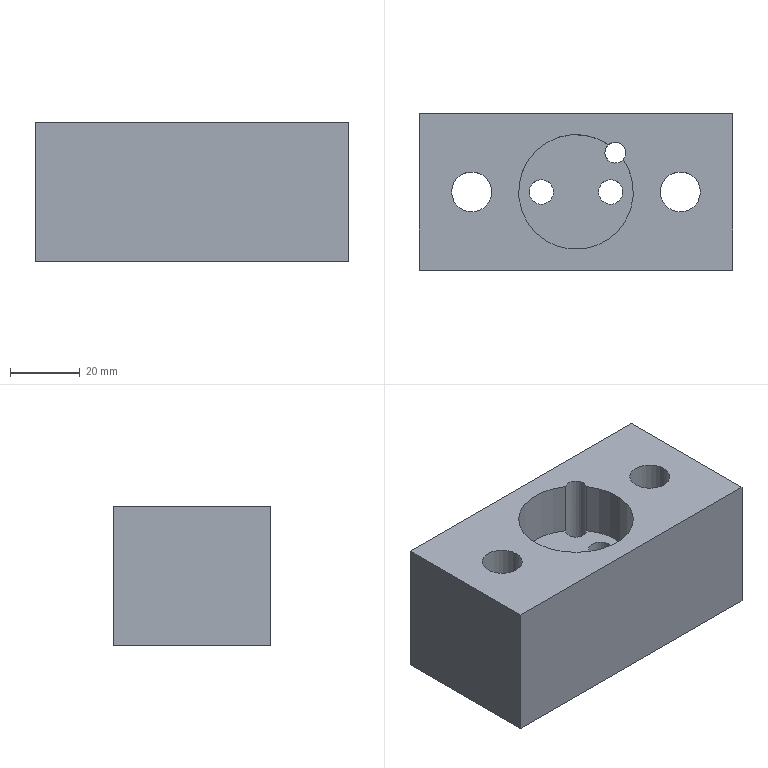Part | NX | features solid 2 | 1 solid | 21 faces | box 90 x 45 x 40 mm | volume 130066 mm3 | plane 11 | cylinder 10 | commonest cylinder face diameters 7 x2 11 x2 11.5 x2 18 x2 6 x1 33 x1
STEP:
#1=CARTESIAN_POINT('',(490.,107.5,-253.));
#2=VERTEX_POINT('',#1);
#3=CARTESIAN_POINT('',(490.,107.5,-213.));
#4=VERTEX_POINT('',#3);
#5=CARTESIAN_POINT('',(490.,107.5,-223.));
#6=DIRECTION('',(0.,0.,1.));
#7=VECTOR('',#6,1000.);
#8=LINE('',#5,#7);
#9=EDGE_CURVE('',#2,#4,#8,.T.);
#10=ORIENTED_EDGE('',*,*,#9,.T.);
#11=CARTESIAN_POINT('',(490.,152.5,-213.));
#12=VERTEX_POINT('',#11);
#13=CARTESIAN_POINT('',(490.,130.,-213.));
#14=DIRECTION('',(0.,1.,0.));
#15=VECTOR('',#14,1000.);
#16=LINE('',#13,#15);
#17=EDGE_CURVE('',#4,#12,#16,.T.);
#18=ORIENTED_EDGE('',*,*,#17,.T.);
#19=CARTESIAN_POINT('',(490.,152.5,-253.));
#20=VERTEX_POINT('',#19);
#21=CARTESIAN_POINT('',(490.,152.5,-223.));
#22=DIRECTION('',(0.,0.,1.));
#23=VECTOR('',#22,1000.);
#24=LINE('',#21,#23);
#25=EDGE_CURVE('',#20,#12,#24,.T.);
#26=ORIENTED_EDGE('',*,*,#25,.F.);
#27=CARTESIAN_POINT('',(490.,130.,-253.));
#28=DIRECTION('',(0.,-1.,0.));
#29=VECTOR('',#28,1000.);
#30=LINE('',#27,#29);
#31=EDGE_CURVE('',#20,#2,#30,.T.);
#32=ORIENTED_EDGE('',*,*,#31,.T.);
#33=EDGE_LOOP('',(#10,#18,#26,#32));
#34=FACE_BOUND('',#33,.T.);
#35=CARTESIAN_POINT('',(490.,130.,-223.));
#36=DIRECTION('',(-1.,0.,0.));
#37=DIRECTION('',(0.,0.,-1.));
#38=AXIS2_PLACEMENT_3D('',#35,#36,#37);
#39=PLANE('',#38);
#40=ADVANCED_FACE('',(#34),#39,.T.);
#41=CARTESIAN_POINT('',(580.,107.5,-253.));
#42=VERTEX_POINT('',#41);
#43=CARTESIAN_POINT('',(580.,107.5,-213.));
#44=VERTEX_POINT('',#43);
#45=CARTESIAN_POINT('',(580.,107.5,-223.));
#46=DIRECTION('',(0.,0.,1.));
#47=VECTOR('',#46,1000.);
#48=LINE('',#45,#47);
#49=EDGE_CURVE('',#42,#44,#48,.T.);
#50=ORIENTED_EDGE('',*,*,#49,.T.);
#51=CARTESIAN_POINT('',(535.,107.5,-213.));
#52=DIRECTION('',(-1.,0.,0.));
#53=VECTOR('',#52,1000.);
#54=LINE('',#51,#53);
#55=EDGE_CURVE('',#44,#4,#54,.T.);
#56=ORIENTED_EDGE('',*,*,#55,.T.);
#57=ORIENTED_EDGE('',*,*,#9,.F.);
#58=CARTESIAN_POINT('',(535.,107.5,-253.));
#59=DIRECTION('',(1.,0.,0.));
#60=VECTOR('',#59,1000.);
#61=LINE('',#58,#60);
#62=EDGE_CURVE('',#2,#42,#61,.T.);
#63=ORIENTED_EDGE('',*,*,#62,.T.);
#64=EDGE_LOOP('',(#50,#56,#57,#63));
#65=FACE_BOUND('',#64,.T.);
#66=CARTESIAN_POINT('',(535.,107.5,-223.));
#67=DIRECTION('',(0.,-1.,0.));
#68=DIRECTION('',(0.,0.,1.));
#69=AXIS2_PLACEMENT_3D('',#66,#67,#68);
#70=PLANE('',#69);
#71=ADVANCED_FACE('',(#65),#70,.T.);
#72=CARTESIAN_POINT('',(580.,152.5,-253.));
#73=VERTEX_POINT('',#72);
#74=CARTESIAN_POINT('',(580.,152.5,-213.));
#75=VERTEX_POINT('',#74);
#76=CARTESIAN_POINT('',(580.,152.5,-223.));
#77=DIRECTION('',(0.,0.,1.));
#78=VECTOR('',#77,1000.);
#79=LINE('',#76,#78);
#80=EDGE_CURVE('',#73,#75,#79,.T.);
#81=ORIENTED_EDGE('',*,*,#80,.T.);
#82=CARTESIAN_POINT('',(580.,130.,-213.));
#83=DIRECTION('',(0.,-1.,0.));
#84=VECTOR('',#83,1000.);
#85=LINE('',#82,#84);
#86=EDGE_CURVE('',#75,#44,#85,.T.);
#87=ORIENTED_EDGE('',*,*,#86,.T.);
#88=ORIENTED_EDGE('',*,*,#49,.F.);
#89=CARTESIAN_POINT('',(580.,130.,-253.));
#90=DIRECTION('',(0.,1.,0.));
#91=VECTOR('',#90,1000.);
#92=LINE('',#89,#91);
#93=EDGE_CURVE('',#42,#73,#92,.T.);
#94=ORIENTED_EDGE('',*,*,#93,.T.);
#95=EDGE_LOOP('',(#81,#87,#88,#94));
#96=FACE_BOUND('',#95,.T.);
#97=CARTESIAN_POINT('',(580.,130.,-223.));
#98=DIRECTION('',(1.,0.,0.));
#99=DIRECTION('',(0.,0.,1.));
#100=AXIS2_PLACEMENT_3D('',#97,#98,#99);
#101=PLANE('',#100);
#102=ADVANCED_FACE('',(#96),#101,.T.);
#103=ORIENTED_EDGE('',*,*,#25,.T.);
#104=CARTESIAN_POINT('',(535.,152.5,-213.));
#105=DIRECTION('',(1.,0.,0.));
#106=VECTOR('',#105,1000.);
#107=LINE('',#104,#106);
#108=EDGE_CURVE('',#12,#75,#107,.T.);
#109=ORIENTED_EDGE('',*,*,#108,.T.);
#110=ORIENTED_EDGE('',*,*,#80,.F.);
#111=CARTESIAN_POINT('',(535.,152.5,-253.));
#112=DIRECTION('',(-1.,0.,0.));
#113=VECTOR('',#112,1000.);
#114=LINE('',#111,#113);
#115=EDGE_CURVE('',#73,#20,#114,.T.);
#116=ORIENTED_EDGE('',*,*,#115,.T.);
#117=EDGE_LOOP('',(#103,#109,#110,#116));
#118=FACE_BOUND('',#117,.T.);
#119=CARTESIAN_POINT('',(535.,152.5,-223.));
#120=DIRECTION('',(0.,1.,0.));
#121=DIRECTION('',(0.,0.,-1.));
#122=AXIS2_PLACEMENT_3D('',#119,#120,#121);
#123=PLANE('',#122);
#124=ADVANCED_FACE('',(#118),#123,.T.);
#125=CARTESIAN_POINT('',(548.435,143.435,-253.));
#126=VERTEX_POINT('',#125);
#127=CARTESIAN_POINT('',(546.314,141.314,-253.));
#128=DIRECTION('',(0.,0.,-1.));
#129=DIRECTION('',(0.7071,0.7071,0.));
#130=AXIS2_PLACEMENT_3D('',#127,#128,#129);
#131=CIRCLE('',#130,3.);
#132=EDGE_CURVE('',#126,#126,#131,.T.);
#133=ORIENTED_EDGE('',*,*,#132,.T.);
#134=EDGE_LOOP('',(#133));
#135=FACE_BOUND('',#134,.T.);
#136=CARTESIAN_POINT('',(544.359,143.589,-213.));
#137=VERTEX_POINT('',#136);
#138=CARTESIAN_POINT('',(548.589,139.359,-213.));
#139=VERTEX_POINT('',#138);
#140=CARTESIAN_POINT('',(546.314,141.314,-213.));
#141=DIRECTION('',(0.,0.,-1.));
#142=DIRECTION('',(1.,0.,0.));
#143=AXIS2_PLACEMENT_3D('',#140,#141,#142);
#144=CIRCLE('',#143,3.);
#145=EDGE_CURVE('',#137,#139,#144,.T.);
#146=ORIENTED_EDGE('',*,*,#145,.F.);
#147=CARTESIAN_POINT('',(544.359,143.589,-228.5));
#148=VERTEX_POINT('',#147);
#149=CARTESIAN_POINT('',(544.359,143.589,-208.));
#150=DIRECTION('',(0.,0.,-1.));
#151=VECTOR('',#150,1000.);
#152=LINE('',#149,#151);
#153=EDGE_CURVE('',#137,#148,#152,.T.);
#154=ORIENTED_EDGE('',*,*,#153,.T.);
#155=CARTESIAN_POINT('',(548.589,139.359,-228.5));
#156=VERTEX_POINT('',#155);
#157=CARTESIAN_POINT('',(546.314,141.314,-228.5));
#158=DIRECTION('',(0.,0.,1.));
#159=DIRECTION('',(-1.,0.,0.));
#160=AXIS2_PLACEMENT_3D('',#157,#158,#159);
#161=CIRCLE('',#160,3.);
#162=EDGE_CURVE('',#148,#156,#161,.T.);
#163=ORIENTED_EDGE('',*,*,#162,.T.);
#164=CARTESIAN_POINT('',(548.589,139.359,-208.));
#165=DIRECTION('',(0.,0.,1.));
#166=VECTOR('',#165,1000.);
#167=LINE('',#164,#166);
#168=EDGE_CURVE('',#156,#139,#167,.T.);
#169=ORIENTED_EDGE('',*,*,#168,.T.);
#170=EDGE_LOOP('',(#146,#154,#163,#169));
#171=FACE_BOUND('',#170,.T.);
#172=CARTESIAN_POINT('',(546.314,141.314,-540.5));
#173=DIRECTION('',(0.,0.,1.));
#174=DIRECTION('',(-0.7071,-0.7071,0.));
#175=AXIS2_PLACEMENT_3D('',#172,#173,#174);
#176=CYLINDRICAL_SURFACE('',#175,3.);
#177=ADVANCED_FACE('',(#135,#171),#176,.F.);
#178=CARTESIAN_POINT('',(570.75,130.,-233.));
#179=VERTEX_POINT('',#178);
#180=CARTESIAN_POINT('',(565.,130.,-233.));
#181=DIRECTION('',(0.,0.,1.));
#182=DIRECTION('',(1.,0.,0.));
#183=AXIS2_PLACEMENT_3D('',#180,#181,#182);
#184=CIRCLE('',#183,5.75);
#185=EDGE_CURVE('',#179,#179,#184,.T.);
#186=ORIENTED_EDGE('',*,*,#185,.F.);
#187=EDGE_LOOP('',(#186));
#188=FACE_BOUND('',#187,.T.);
#189=CARTESIAN_POINT('',(570.75,130.,-213.));
#190=VERTEX_POINT('',#189);
#191=CARTESIAN_POINT('',(565.,130.,-213.));
#192=DIRECTION('',(0.,0.,-1.));
#193=DIRECTION('',(1.,0.,0.));
#194=AXIS2_PLACEMENT_3D('',#191,#192,#193);
#195=CIRCLE('',#194,5.75);
#196=EDGE_CURVE('',#190,#190,#195,.T.);
#197=ORIENTED_EDGE('',*,*,#196,.F.);
#198=EDGE_LOOP('',(#197));
#199=FACE_BOUND('',#198,.T.);
#200=CARTESIAN_POINT('',(565.,130.,-233.));
#201=DIRECTION('',(0.,0.,1.));
#202=DIRECTION('',(-1.,0.,0.));
#203=AXIS2_PLACEMENT_3D('',#200,#201,#202);
#204=CYLINDRICAL_SURFACE('',#203,5.75);
#205=ADVANCED_FACE('',(#188,#199),#204,.F.);
#206=CARTESIAN_POINT('',(510.75,130.,-233.));
#207=VERTEX_POINT('',#206);
#208=CARTESIAN_POINT('',(505.,130.,-233.));
#209=DIRECTION('',(0.,0.,-1.));
#210=DIRECTION('',(1.,0.,0.));
#211=AXIS2_PLACEMENT_3D('',#208,#209,#210);
#212=CIRCLE('',#211,5.75);
#213=EDGE_CURVE('',#207,#207,#212,.T.);
#214=ORIENTED_EDGE('',*,*,#213,.T.);
#215=EDGE_LOOP('',(#214));
#216=FACE_BOUND('',#215,.T.);
#217=CARTESIAN_POINT('',(510.75,130.,-213.));
#218=VERTEX_POINT('',#217);
#219=CARTESIAN_POINT('',(505.,130.,-213.));
#220=DIRECTION('',(0.,0.,-1.));
#221=DIRECTION('',(1.,0.,0.));
#222=AXIS2_PLACEMENT_3D('',#219,#220,#221);
#223=CIRCLE('',#222,5.75);
#224=EDGE_CURVE('',#218,#218,#223,.T.);
#225=ORIENTED_EDGE('',*,*,#224,.F.);
#226=EDGE_LOOP('',(#225));
#227=FACE_BOUND('',#226,.T.);
#228=CARTESIAN_POINT('',(505.,130.,-233.));
#229=DIRECTION('',(0.,0.,1.));
#230=DIRECTION('',(1.,0.,0.));
#231=AXIS2_PLACEMENT_3D('',#228,#229,#230);
#232=CYLINDRICAL_SURFACE('',#231,5.75);
#233=ADVANCED_FACE('',(#216,#227),#232,.F.);
#234=CARTESIAN_POINT('',(535.,130.,-213.));
#235=DIRECTION('',(0.,0.,-1.));
#236=DIRECTION('',(1.,0.,0.));
#237=AXIS2_PLACEMENT_3D('',#234,#235,#236);
#238=CIRCLE('',#237,16.5);
#239=EDGE_CURVE('',#139,#137,#238,.T.);
#240=ORIENTED_EDGE('',*,*,#239,.F.);
#241=ORIENTED_EDGE('',*,*,#168,.F.);
#242=CARTESIAN_POINT('',(535.,130.,-228.5));
#243=DIRECTION('',(0.,0.,-1.));
#244=DIRECTION('',(-1.,0.,0.));
#245=AXIS2_PLACEMENT_3D('',#242,#243,#244);
#246=CIRCLE('',#245,16.5);
#247=EDGE_CURVE('',#156,#148,#246,.T.);
#248=ORIENTED_EDGE('',*,*,#247,.T.);
#249=ORIENTED_EDGE('',*,*,#153,.F.);
#250=EDGE_LOOP('',(#240,#241,#248,#249));
#251=FACE_BOUND('',#250,.T.);
#252=CARTESIAN_POINT('',(535.,130.,-156.7));
#253=DIRECTION('',(0.,0.,-1.));
#254=DIRECTION('',(0.,-1.,0.));
#255=AXIS2_PLACEMENT_3D('',#252,#253,#254);
#256=CYLINDRICAL_SURFACE('',#255,16.5);
#257=ADVANCED_FACE('',(#251),#256,.F.);
#258=CARTESIAN_POINT('',(550.5,130.,-239.));
#259=VERTEX_POINT('',#258);
#260=CARTESIAN_POINT('',(545.,130.,-239.));
#261=DIRECTION('',(0.,0.,1.));
#262=DIRECTION('',(1.,0.,0.));
#263=AXIS2_PLACEMENT_3D('',#260,#261,#262);
#264=CIRCLE('',#263,5.5);
#265=EDGE_CURVE('',#259,#259,#264,.T.);
#266=ORIENTED_EDGE('',*,*,#265,.T.);
#267=EDGE_LOOP('',(#266));
#268=FACE_BOUND('',#267,.T.);
#269=CARTESIAN_POINT('',(550.5,130.,-253.));
#270=VERTEX_POINT('',#269);
#271=CARTESIAN_POINT('',(545.,130.,-253.));
#272=DIRECTION('',(0.,0.,1.));
#273=DIRECTION('',(1.,0.,0.));
#274=AXIS2_PLACEMENT_3D('',#271,#272,#273);
#275=CIRCLE('',#274,5.5);
#276=EDGE_CURVE('',#270,#270,#275,.T.);
#277=ORIENTED_EDGE('',*,*,#276,.F.);
#278=EDGE_LOOP('',(#277));
#279=FACE_BOUND('',#278,.T.);
#280=CARTESIAN_POINT('',(545.,130.,42.));
#281=DIRECTION('',(0.,0.,-1.));
#282=DIRECTION('',(1.,0.,0.));
#283=AXIS2_PLACEMENT_3D('',#280,#281,#282);
#284=CYLINDRICAL_SURFACE('',#283,5.5);
#285=ADVANCED_FACE('',(#268,#279),#284,.F.);
#286=CARTESIAN_POINT('',(496.,130.,-253.));
#287=VERTEX_POINT('',#286);
#288=CARTESIAN_POINT('',(505.,130.,-253.));
#289=DIRECTION('',(0.,0.,-1.));
#290=DIRECTION('',(-1.,0.,0.));
#291=AXIS2_PLACEMENT_3D('',#288,#289,#290);
#292=CIRCLE('',#291,9.);
#293=EDGE_CURVE('',#287,#287,#292,.T.);
#294=ORIENTED_EDGE('',*,*,#293,.T.);
#295=EDGE_LOOP('',(#294));
#296=FACE_BOUND('',#295,.T.);
#297=CARTESIAN_POINT('',(514.,130.,-233.));
#298=VERTEX_POINT('',#297);
#299=CARTESIAN_POINT('',(505.,130.,-233.));
#300=DIRECTION('',(0.,0.,-1.));
#301=DIRECTION('',(1.,0.,0.));
#302=AXIS2_PLACEMENT_3D('',#299,#300,#301);
#303=CIRCLE('',#302,9.);
#304=EDGE_CURVE('',#298,#298,#303,.T.);
#305=ORIENTED_EDGE('',*,*,#304,.F.);
#306=EDGE_LOOP('',(#305));
#307=FACE_BOUND('',#306,.T.);
#308=CARTESIAN_POINT('',(505.,130.,-233.));
#309=DIRECTION('',(0.,0.,1.));
#310=DIRECTION('',(1.,0.,0.));
#311=AXIS2_PLACEMENT_3D('',#308,#309,#310);
#312=CYLINDRICAL_SURFACE('',#311,9.);
#313=ADVANCED_FACE('',(#296,#307),#312,.F.);
#314=CARTESIAN_POINT('',(556.,130.,-253.));
#315=VERTEX_POINT('',#314);
#316=CARTESIAN_POINT('',(565.,130.,-253.));
#317=DIRECTION('',(0.,0.,1.));
#318=DIRECTION('',(-1.,0.,0.));
#319=AXIS2_PLACEMENT_3D('',#316,#317,#318);
#320=CIRCLE('',#319,9.);
#321=EDGE_CURVE('',#315,#315,#320,.T.);
#322=ORIENTED_EDGE('',*,*,#321,.F.);
#323=EDGE_LOOP('',(#322));
#324=FACE_BOUND('',#323,.T.);
#325=CARTESIAN_POINT('',(574.,130.,-233.));
#326=VERTEX_POINT('',#325);
#327=CARTESIAN_POINT('',(565.,130.,-233.));
#328=DIRECTION('',(0.,0.,1.));
#329=DIRECTION('',(1.,0.,0.));
#330=AXIS2_PLACEMENT_3D('',#327,#328,#329);
#331=CIRCLE('',#330,9.);
#332=EDGE_CURVE('',#326,#326,#331,.T.);
#333=ORIENTED_EDGE('',*,*,#332,.T.);
#334=EDGE_LOOP('',(#333));
#335=FACE_BOUND('',#334,.T.);
#336=CARTESIAN_POINT('',(565.,130.,-233.));
#337=DIRECTION('',(0.,0.,1.));
#338=DIRECTION('',(-1.,0.,0.));
#339=AXIS2_PLACEMENT_3D('',#336,#337,#338);
#340=CYLINDRICAL_SURFACE('',#339,9.);
#341=ADVANCED_FACE('',(#324,#335),#340,.F.);
#342=CARTESIAN_POINT('',(530.5,130.,-253.));
#343=VERTEX_POINT('',#342);
#344=CARTESIAN_POINT('',(525.,130.,-253.));
#345=DIRECTION('',(0.,0.,-1.));
#346=DIRECTION('',(1.,0.,0.));
#347=AXIS2_PLACEMENT_3D('',#344,#345,#346);
#348=CIRCLE('',#347,5.5);
#349=EDGE_CURVE('',#343,#343,#348,.T.);
#350=ORIENTED_EDGE('',*,*,#349,.F.);
#351=EDGE_LOOP('',(#350));
#352=FACE_BOUND('',#351,.T.);
#353=ORIENTED_EDGE('',*,*,#321,.T.);
#354=EDGE_LOOP('',(#353));
#355=FACE_BOUND('',#354,.T.);
#356=ORIENTED_EDGE('',*,*,#132,.F.);
#357=EDGE_LOOP('',(#356));
#358=FACE_BOUND('',#357,.T.);
#359=ORIENTED_EDGE('',*,*,#31,.F.);
#360=ORIENTED_EDGE('',*,*,#115,.F.);
#361=ORIENTED_EDGE('',*,*,#93,.F.);
#362=ORIENTED_EDGE('',*,*,#62,.F.);
#363=EDGE_LOOP('',(#359,#360,#361,#362));
#364=FACE_BOUND('',#363,.T.);
#365=ORIENTED_EDGE('',*,*,#293,.F.);
#366=EDGE_LOOP('',(#365));
#367=FACE_BOUND('',#366,.T.);
#368=ORIENTED_EDGE('',*,*,#276,.T.);
#369=EDGE_LOOP('',(#368));
#370=FACE_BOUND('',#369,.T.);
#371=CARTESIAN_POINT('',(535.,130.,-253.));
#372=DIRECTION('',(0.,0.,-1.));
#373=DIRECTION('',(1.,0.,0.));
#374=AXIS2_PLACEMENT_3D('',#371,#372,#373);
#375=PLANE('',#374);
#376=ADVANCED_FACE('',(#352,#355,#358,#364,#367,#370),#375,.T.);
#377=CARTESIAN_POINT('',(530.5,130.,-239.));
#378=VERTEX_POINT('',#377);
#379=CARTESIAN_POINT('',(525.,130.,-239.));
#380=DIRECTION('',(0.,0.,1.));
#381=DIRECTION('',(1.,0.,0.));
#382=AXIS2_PLACEMENT_3D('',#379,#380,#381);
#383=CIRCLE('',#382,5.5);
#384=EDGE_CURVE('',#378,#378,#383,.T.);
#385=ORIENTED_EDGE('',*,*,#384,.T.);
#386=EDGE_LOOP('',(#385));
#387=FACE_BOUND('',#386,.T.);
#388=ORIENTED_EDGE('',*,*,#349,.T.);
#389=EDGE_LOOP('',(#388));
#390=FACE_BOUND('',#389,.T.);
#391=CARTESIAN_POINT('',(525.,130.,42.));
#392=DIRECTION('',(0.,0.,-1.));
#393=DIRECTION('',(1.,0.,0.));
#394=AXIS2_PLACEMENT_3D('',#391,#392,#393);
#395=CYLINDRICAL_SURFACE('',#394,5.5);
#396=ADVANCED_FACE('',(#387,#390),#395,.F.);
#397=CARTESIAN_POINT('',(528.5,130.,-239.));
#398=VERTEX_POINT('',#397);
#399=CARTESIAN_POINT('',(525.,130.,-239.));
#400=DIRECTION('',(0.,0.,-1.));
#401=DIRECTION('',(1.,0.,0.));
#402=AXIS2_PLACEMENT_3D('',#399,#400,#401);
#403=CIRCLE('',#402,3.5);
#404=EDGE_CURVE('',#398,#398,#403,.T.);
#405=ORIENTED_EDGE('',*,*,#404,.F.);
#406=EDGE_LOOP('',(#405));
#407=FACE_BOUND('',#406,.T.);
#408=ORIENTED_EDGE('',*,*,#384,.F.);
#409=EDGE_LOOP('',(#408));
#410=FACE_BOUND('',#409,.T.);
#411=CARTESIAN_POINT('',(535.,129.476,-239.));
#412=DIRECTION('',(0.,0.,-1.));
#413=DIRECTION('',(1.,0.,0.));
#414=AXIS2_PLACEMENT_3D('',#411,#412,#413);
#415=PLANE('',#414);
#416=ADVANCED_FACE('',(#407,#410),#415,.T.);
#417=CARTESIAN_POINT('',(548.5,130.,-239.));
#418=VERTEX_POINT('',#417);
#419=CARTESIAN_POINT('',(545.,130.,-239.));
#420=DIRECTION('',(0.,0.,-1.));
#421=DIRECTION('',(1.,0.,0.));
#422=AXIS2_PLACEMENT_3D('',#419,#420,#421);
#423=CIRCLE('',#422,3.5);
#424=EDGE_CURVE('',#418,#418,#423,.T.);
#425=ORIENTED_EDGE('',*,*,#424,.F.);
#426=EDGE_LOOP('',(#425));
#427=FACE_BOUND('',#426,.T.);
#428=ORIENTED_EDGE('',*,*,#265,.F.);
#429=EDGE_LOOP('',(#428));
#430=FACE_BOUND('',#429,.T.);
#431=CARTESIAN_POINT('',(535.,129.476,-239.));
#432=DIRECTION('',(0.,0.,-1.));
#433=DIRECTION('',(1.,0.,0.));
#434=AXIS2_PLACEMENT_3D('',#431,#432,#433);
#435=PLANE('',#434);
#436=ADVANCED_FACE('',(#427,#430),#435,.T.);
#437=CARTESIAN_POINT('',(541.5,130.,-228.5));
#438=VERTEX_POINT('',#437);
#439=CARTESIAN_POINT('',(545.,130.,-228.5));
#440=DIRECTION('',(0.,0.,1.));
#441=DIRECTION('',(-1.,0.,0.));
#442=AXIS2_PLACEMENT_3D('',#439,#440,#441);
#443=CIRCLE('',#442,3.5);
#444=EDGE_CURVE('',#438,#438,#443,.T.);
#445=ORIENTED_EDGE('',*,*,#444,.T.);
#446=EDGE_LOOP('',(#445));
#447=FACE_BOUND('',#446,.T.);
#448=ORIENTED_EDGE('',*,*,#424,.T.);
#449=EDGE_LOOP('',(#448));
#450=FACE_BOUND('',#449,.T.);
#451=CARTESIAN_POINT('',(545.,130.,42.));
#452=DIRECTION('',(0.,0.,-1.));
#453=DIRECTION('',(1.,0.,0.));
#454=AXIS2_PLACEMENT_3D('',#451,#452,#453);
#455=CYLINDRICAL_SURFACE('',#454,3.5);
#456=ADVANCED_FACE('',(#447,#450),#455,.F.);
#457=CARTESIAN_POINT('',(521.5,130.,-228.5));
#458=VERTEX_POINT('',#457);
#459=CARTESIAN_POINT('',(525.,130.,-228.5));
#460=DIRECTION('',(0.,0.,1.));
#461=DIRECTION('',(-1.,0.,0.));
#462=AXIS2_PLACEMENT_3D('',#459,#460,#461);
#463=CIRCLE('',#462,3.5);
#464=EDGE_CURVE('',#458,#458,#463,.T.);
#465=ORIENTED_EDGE('',*,*,#464,.T.);
#466=EDGE_LOOP('',(#465));
#467=FACE_BOUND('',#466,.T.);
#468=ORIENTED_EDGE('',*,*,#404,.T.);
#469=EDGE_LOOP('',(#468));
#470=FACE_BOUND('',#469,.T.);
#471=CARTESIAN_POINT('',(525.,130.,42.));
#472=DIRECTION('',(0.,0.,-1.));
#473=DIRECTION('',(1.,0.,0.));
#474=AXIS2_PLACEMENT_3D('',#471,#472,#473);
#475=CYLINDRICAL_SURFACE('',#474,3.5);
#476=ADVANCED_FACE('',(#467,#470),#475,.F.);
#477=ORIENTED_EDGE('',*,*,#185,.T.);
#478=EDGE_LOOP('',(#477));
#479=FACE_BOUND('',#478,.T.);
#480=ORIENTED_EDGE('',*,*,#332,.F.);
#481=EDGE_LOOP('',(#480));
#482=FACE_BOUND('',#481,.T.);
#483=CARTESIAN_POINT('',(565.,130.,-233.));
#484=DIRECTION('',(0.,0.,1.));
#485=DIRECTION('',(-1.,0.,0.));
#486=AXIS2_PLACEMENT_3D('',#483,#484,#485);
#487=PLANE('',#486);
#488=ADVANCED_FACE('',(#479,#482),#487,.F.);
#489=ORIENTED_EDGE('',*,*,#213,.F.);
#490=EDGE_LOOP('',(#489));
#491=FACE_BOUND('',#490,.T.);
#492=ORIENTED_EDGE('',*,*,#304,.T.);
#493=EDGE_LOOP('',(#492));
#494=FACE_BOUND('',#493,.T.);
#495=CARTESIAN_POINT('',(505.,130.,-233.));
#496=DIRECTION('',(0.,0.,1.));
#497=DIRECTION('',(1.,0.,0.));
#498=AXIS2_PLACEMENT_3D('',#495,#496,#497);
#499=PLANE('',#498);
#500=ADVANCED_FACE('',(#491,#494),#499,.F.);
#501=ORIENTED_EDGE('',*,*,#444,.F.);
#502=EDGE_LOOP('',(#501));
#503=FACE_BOUND('',#502,.T.);
#504=ORIENTED_EDGE('',*,*,#464,.F.);
#505=EDGE_LOOP('',(#504));
#506=FACE_BOUND('',#505,.T.);
#507=ORIENTED_EDGE('',*,*,#247,.F.);
#508=ORIENTED_EDGE('',*,*,#162,.F.);
#509=EDGE_LOOP('',(#507,#508));
#510=FACE_BOUND('',#509,.T.);
#511=CARTESIAN_POINT('',(542.475,130.,-228.5));
#512=DIRECTION('',(0.,0.,-1.));
#513=DIRECTION('',(1.,0.,0.));
#514=AXIS2_PLACEMENT_3D('',#511,#512,#513);
#515=PLANE('',#514);
#516=ADVANCED_FACE('',(#503,#506,#510),#515,.F.);
#517=ORIENTED_EDGE('',*,*,#17,.F.);
#518=ORIENTED_EDGE('',*,*,#55,.F.);
#519=ORIENTED_EDGE('',*,*,#86,.F.);
#520=ORIENTED_EDGE('',*,*,#108,.F.);
#521=EDGE_LOOP('',(#517,#518,#519,#520));
#522=FACE_BOUND('',#521,.T.);
#523=ORIENTED_EDGE('',*,*,#224,.T.);
#524=EDGE_LOOP('',(#523));
#525=FACE_BOUND('',#524,.T.);
#526=ORIENTED_EDGE('',*,*,#239,.T.);
#527=ORIENTED_EDGE('',*,*,#145,.T.);
#528=EDGE_LOOP('',(#526,#527));
#529=FACE_BOUND('',#528,.T.);
#530=ORIENTED_EDGE('',*,*,#196,.T.);
#531=EDGE_LOOP('',(#530));
#532=FACE_BOUND('',#531,.T.);
#533=CARTESIAN_POINT('',(142.706,0.,-213.));
#534=DIRECTION('',(0.,0.,1.));
#535=DIRECTION('',(-1.,0.,0.));
#536=AXIS2_PLACEMENT_3D('',#533,#534,#535);
#537=PLANE('',#536);
#538=ADVANCED_FACE('',(#522,#525,#529,#532),#537,.T.);
#539=CLOSED_SHELL('',(#40,#71,#102,#124,#177,#205,#233,#257,#285,#313,#341,#376,#396,#416,#436,#456,#476,#488,#500,#516,#538));
#540=MANIFOLD_SOLID_BREP('',#539);
#541=(LENGTH_UNIT()NAMED_UNIT(*)SI_UNIT(.MILLI.,.METRE.));
#542=UNCERTAINTY_MEASURE_WITH_UNIT(LENGTH_MEASURE(0.00001),#541,'','');
#543=(NAMED_UNIT(*)PLANE_ANGLE_UNIT()SI_UNIT($,.RADIAN.));
#544=(NAMED_UNIT(*)SI_UNIT($,.STERADIAN.)SOLID_ANGLE_UNIT());
#545=(GEOMETRIC_REPRESENTATION_CONTEXT(3)GLOBAL_UNCERTAINTY_ASSIGNED_CONTEXT((#542))GLOBAL_UNIT_ASSIGNED_CONTEXT((#541,#543,#544))REPRESENTATION_CONTEXT('',''));
#546=ADVANCED_BREP_SHAPE_REPRESENTATION('',(#540),#545);